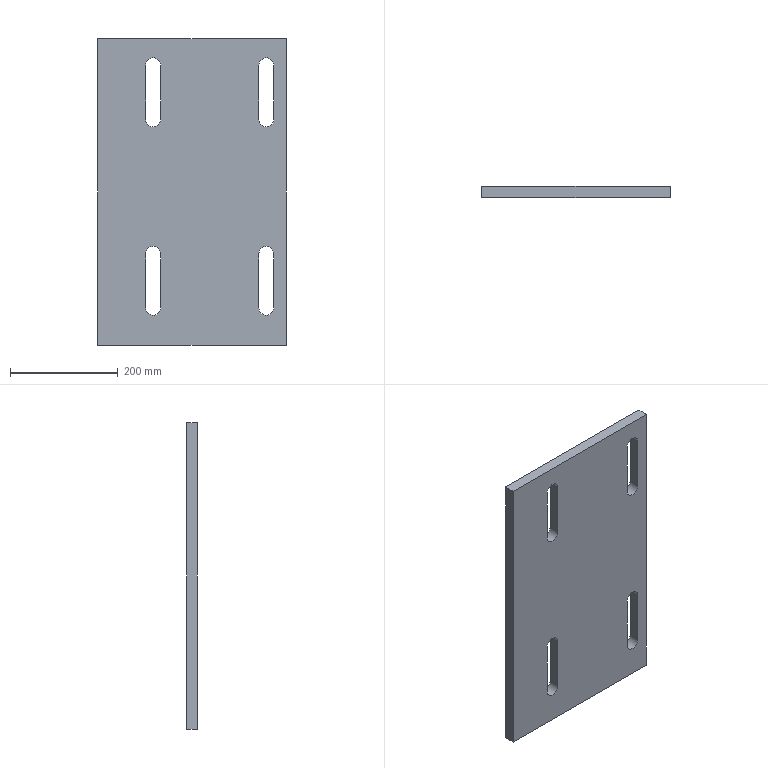Part | STEP file | Input 75 | 1 solid | 22 faces | box 350 x 20 x 570 mm | volume 3716740 mm3 | plane 14 | cylinder 8 | commonest cylinder face diameters 28 x8